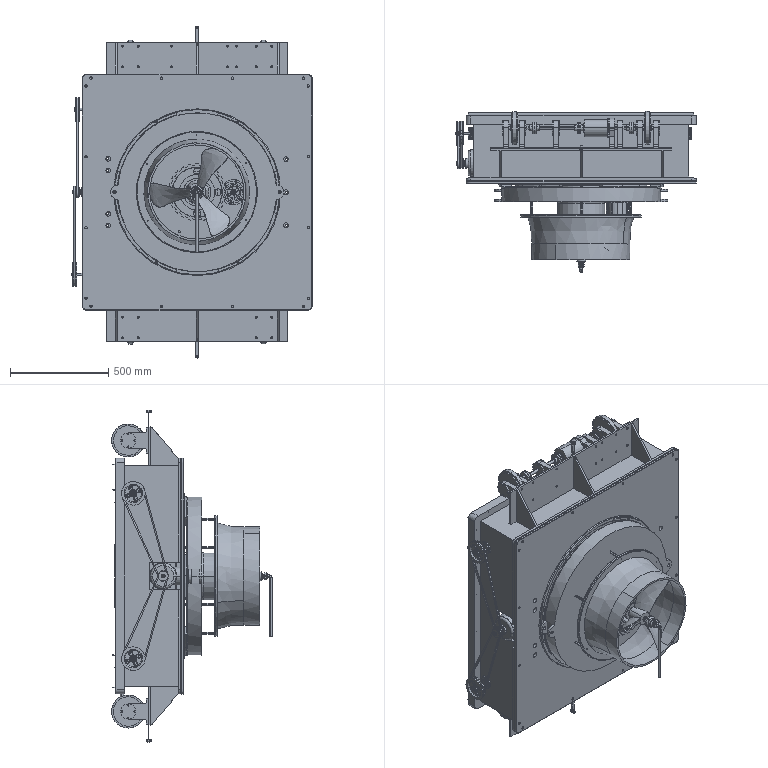Part | NX | features BREP 907 | 1251 solids | 12935 faces | volume 106230951 mm3 | cylinder 6144 | plane 3715 | sphere 1724 | cone 616 | torus 465 | spline 271 | commonest cylinder face diameters 2 x2680 6 x417 10 x293 8 x225 12 x201 5 x200